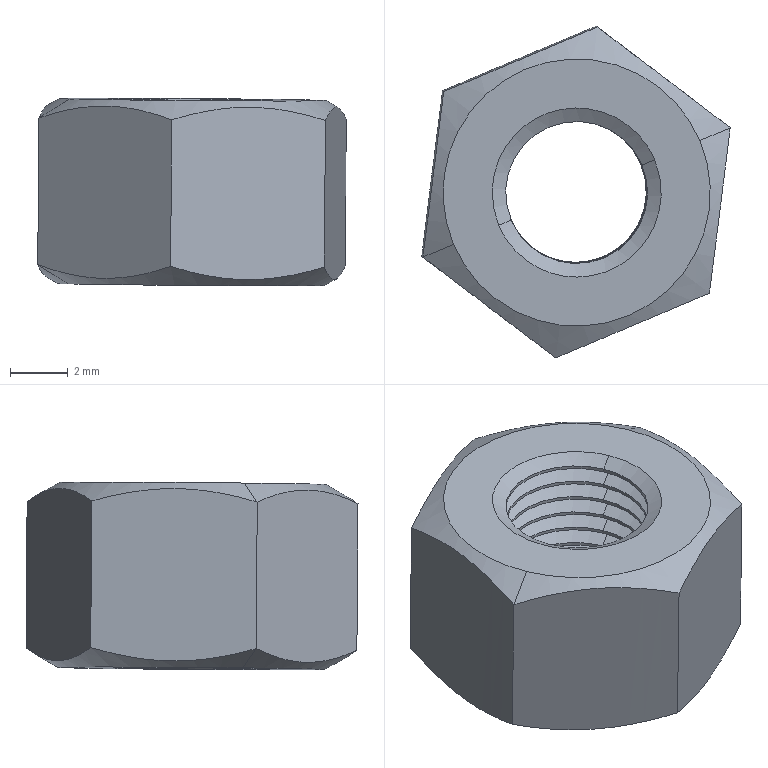Part | STEP file | PN_0019_Default<As Machined> | 1 solid | 72 faces | box 10.681 x 11.495 x 6.499 mm | volume 404.351 mm3 | cone 44 | cylinder 20 | plane 8 | commonest cylinder face diameters 4.917 x20